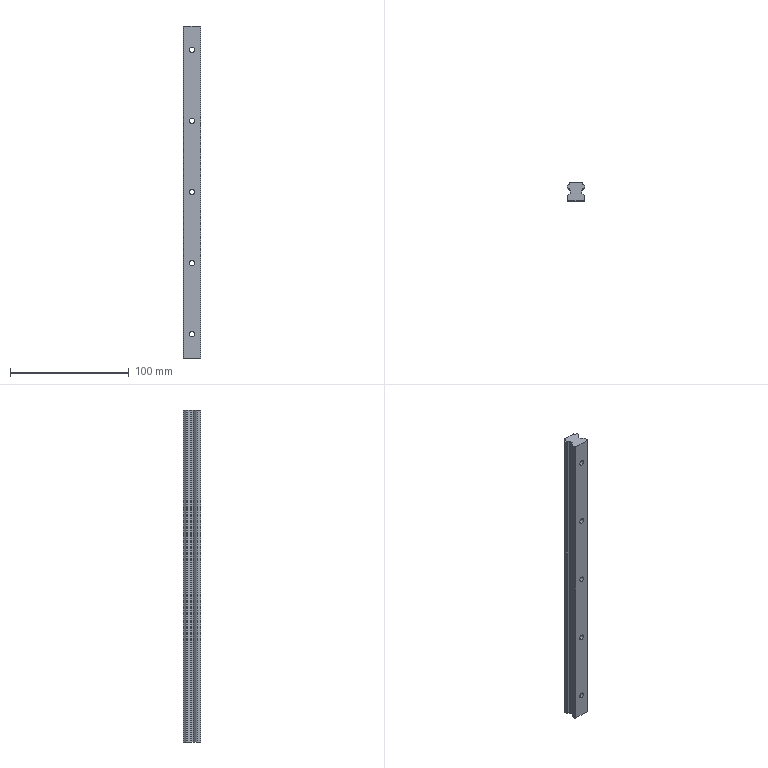Part | STEP file | HGR15 | 1 solid | 61 faces | box 15 x 15 x 280 mm | volume 51471 mm3 | cylinder 34 | plane 27 | commonest cylinder face diameters 4.5 x10 7.5 x10 0.8 x8 3.24 x4 2 x2